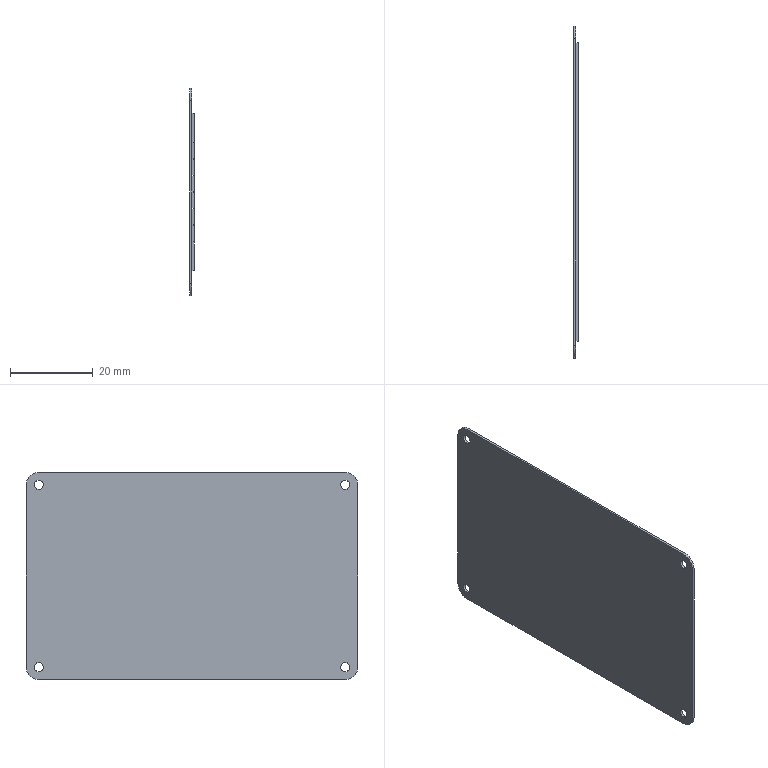Part | SolidWorks | features BaseBody 1 | 1 solid | 4520 faces | volume 3306 mm3 | plane 3263 | spline 793 | cylinder 464 | commonest cylinder face diameters 1.863 x67 2.661 x13 2.2 x8 1.781 x4 4.299 x4 4.634 x4